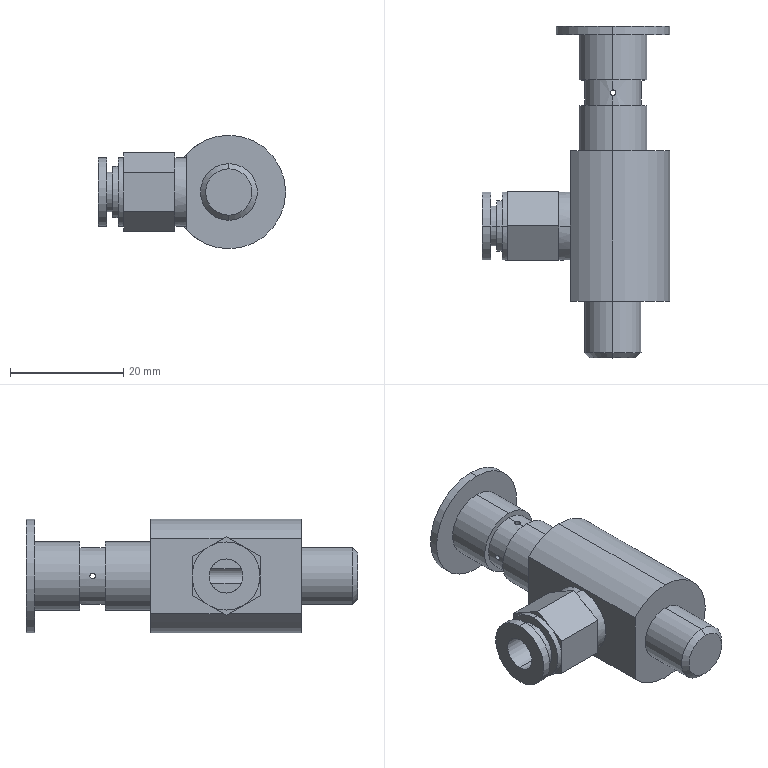Part | SolidWorks | features BaseBody 1 | 1 solid | 74 faces | box 33 x 58.5 x 20 mm | volume 11826 mm3 | cylinder 36 | plane 32 | cone 6 | commonest cylinder face diameters 12 x10 1 x8 20 x5 10 x4 3.242 x3 6 x2